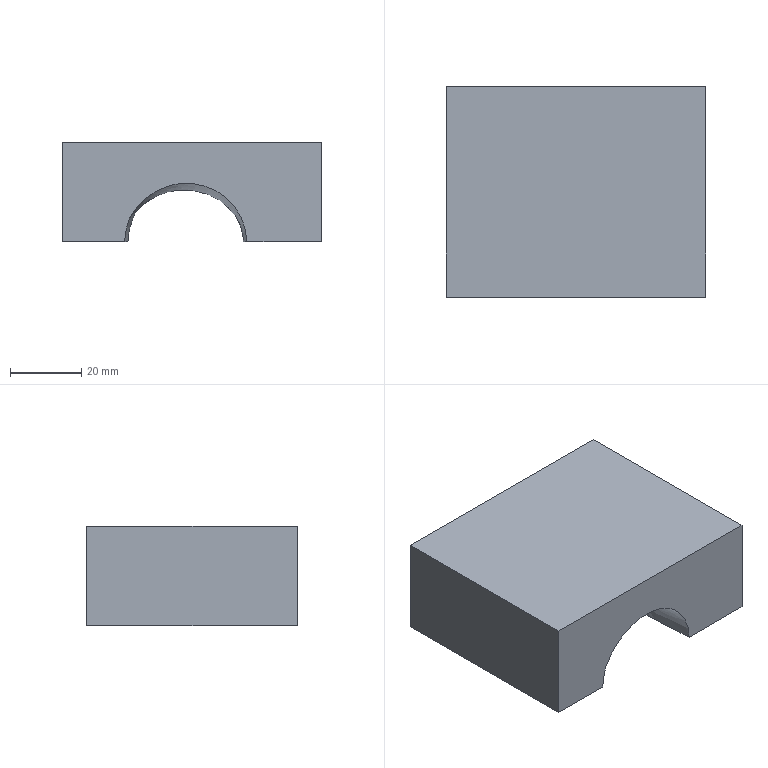NC program | NX | posted with a generic post | part box 72.744 x 59.015 x 27.972 mm
Lines 1756 to 2547 of 95982:
(FIXED_CONTOUR , TOOL : R2)
N3474 T11 M6
N3476 G54
N3478 G17 G0 G90 X13.244 Y-31.06 S9500 M3
N3480 G43 Z30. H11
N3482 Z5.2
N3484 G94 G1 Z0.147 F1000.
N3486 X13.257 Y-31.089
N3488 X13.248 Y-31.119
N3490 X13.223 Y-31.137
N3492 X13.217 Y-31.144 Z-0.024 F3000.
N3494 X13.192 Y-31.168 Z-1.496
N3496 X13.168 Y-31.192 Z-2.478
N3498 X13.124 Y-31.237 Z-3.072
N3500 X13.105 Y-31.256 Z-3.228
N3502 X13.073 Y-31.288 Z-3.473
N3504 X13.053 Y-31.289 Z-3.655
N3506 X13.028 Y-31.29 Z-3.843
N3508 X13.008 Z-3.965
N3510 X13.034 Y-31.263 Z-3.831
N3512 X13.053 Y-31.245 Z-3.714
N3514 X13.11 Y-31.188 Z-3.284
N3516 X13.134 Y-31.163 Z-3.109
N3518 X13.183 Y-31.115 Z-2.494
N3520 X13.208 Y-31.09 Z-1.499
N3522 X13.234 Y-31.064 Z0.072
N3524 X13.237 Y-31.061 Z0.149
N3526 X13.242 Y-31.031 Z0.15
N3528 X13.214 Y-31.059 Z-1.5
N3530 X13.188 Y-31.085 Z-2.501
N3532 X13.139 Y-31.134 Z-3.123
N3534 X13.087 Y-31.186 Z-3.491
N3536 X13.054 Y-31.22 Z-3.747
N3538 X13.042 Y-31.231 Z-3.817
N3540 X12.983 Y-31.29 Z-4.119
N3542 X12.959 Y-31.291 Z-4.273
N3544 X13.054 Y-31.196 Z-3.778
N3546 X13.144 Y-31.107 Z-3.135
N3548 X13.193 Y-31.057 Z-2.507
N3550 X13.219 Y-31.031 Z-1.501
N3552 X13.247 Y-31.004 Z0.151
N3554 X13.251 Y-30.981
N3556 X13.223 Y-31.009 Z-1.553
N3558 X13.198 Y-31.034 Z-2.512
N3560 X13.147 Y-31.084 Z-3.146
N3562 X13.055 Y-31.177 Z-3.799
N3564 X12.94 Y-31.292 Z-4.4
N3566 X12.921 Z-4.503
N3568 X12.947 Y-31.265 Z-4.388
N3570 X13.057 Y-31.156 Z-3.812
N3572 X13.151 Y-31.062 Z-3.156
N3574 X13.202 Y-31.011 Z-2.517
N3576 X13.229 Y-30.984 Z-1.512
N3578 X13.255 Y-30.957 Z0.152
N3580 X13.26 Y-30.933
N3582 X13.233 Y-30.96 Z-1.528
N3584 X13.206 Y-30.987 Z-2.524
N3586 X13.155 Y-31.038 Z-3.167
N3588 X13.115 Y-31.078 Z-3.449
N3590 X13.06 Y-31.133 Z-3.825
N3592 X12.957 Y-31.236 Z-4.361
N3594 X12.901 Y-31.292 Z-4.606
N3596 X12.88 Y-31.291 Z-4.713
N3598 X12.902 Y-31.27 Z-4.628
N3600 X12.969 Y-31.203 Z-4.331
N3602 X13.062 Y-31.109 Z-3.84
N3604 X13.159 Y-31.013 Z-3.179
N3606 X13.211 Y-30.96 Z-2.532
N3608 X13.238 Y-30.933 Z-1.546
N3610 X13.265 Y-30.906 Z0.153
N3612 X13.271 Y-30.877 Z0.154
N3614 X13.243 Y-30.904 Z-1.565
N3616 X13.222 Y-30.926 Z-2.383
N3618 X13.216 Y-30.932 Z-2.54
N3620 X13.162 Y-30.985 Z-3.197
N3622 X13.065 Y-31.083 Z-3.856
N3624 X12.978 Y-31.169 Z-4.312
N3626 X12.902 Y-31.246 Z-4.653
N3628 X12.89 Y-31.257 Z-4.689
N3630 X12.856 Y-31.292 Z-4.831
N3632 X12.83 Y-31.293 Z-4.96
N3634 X12.884 Y-31.238 Z-4.737
N3636 X12.902 Y-31.22 Z-4.68
N3638 X12.98 Y-31.142 Z-4.334
N3640 X13.068 Y-31.054 Z-3.873
N3642 X13.165 Y-30.957 Z-3.222
N3644 X13.172 Y-30.95 Z-3.167
N3646 X13.222 Y-30.9 Z-2.55
N3648 X13.23 Y-30.892 Z-2.32
N3650 X13.249 Y-30.873 Z-1.586
N3652 X13.277 Y-30.845 Z0.155
N3654 X13.283 Y-30.811
N3656 X13.256 Y-30.839 Z-1.608
N3658 X13.239 Y-30.856 Z-2.251
N3660 X13.228 Y-30.867 Z-2.56
N3662 X13.18 Y-30.915 Z-3.153
N3664 X13.168 Y-30.926 Z-3.25
N3666 X13.072 Y-31.023 Z-3.892
N3668 X12.982 Y-31.113 Z-4.358
N3670 X12.902 Y-31.193 Z-4.709
N3672 X12.877 Y-31.218 Z-4.789
N3674 X12.801 Y-31.293 Z-5.099
N3676 X12.768 Z-5.243
N3678 X12.802 Y-31.259 Z-5.124
N3680 X12.868 Y-31.193 Z-4.852
N3682 X12.902 Y-31.159 Z-4.744
N3684 X12.984 Y-31.078 Z-4.387
N3686 X13.08 Y-30.981 Z-3.891
N3688 X13.172 Y-30.889 Z-3.283
N3690 X13.19 Y-30.872 Z-3.137
N3692 X13.235 Y-30.826 Z-2.573
N3694 X13.249 Y-30.812 Z-2.168
N3696 X13.263 Y-30.798 Z-1.635
N3698 X13.291 Y-30.77 Z0.156
N3700 X13.298 Y-30.733 Z0.157
N3702 X13.27 Y-30.761 Z-1.66
N3704 X13.259 Y-30.773 Z-2.094
N3706 X13.242 Y-30.79 Z-2.584
N3708 X13.198 Y-30.833 Z-3.122
N3710 X13.175 Y-30.856 Z-3.312
N3712 X13.094 Y-30.938 Z-3.851
N3714 X13.078 Y-30.954 Z-3.945
N3716 X12.985 Y-31.046 Z-4.413
N3718 X12.902 Y-31.13 Z-4.772
N3720 X12.861 Y-31.171 Z-4.908
N3722 X12.802 Y-31.229 Z-5.149
N3724 X12.738 Y-31.293 Z-5.371
N3726 X12.71 Z-5.487
N3728 X12.735 Y-31.268 Z-5.408
N3730 X12.802 Y-31.201 Z-5.173
N3732 X12.854 Y-31.149 Z-4.961
N3734 X12.877 Y-31.126 Z-4.887
N3736 X12.902 Y-31.101 Z-4.799
N3738 X12.987 Y-31.016 Z-4.438
N3740 X13.08 Y-30.923 Z-3.971
N3742 X13.107 Y-30.896 Z-3.813
N3744 X13.178 Y-30.825 Z-3.341
N3746 X13.206 Y-30.797 Z-3.108
N3748 X13.248 Y-30.755 Z-2.595
N3750 X13.268 Y-30.735 Z-2.023
N3752 X13.277 Y-30.726 Z-1.683
N3754 X13.305 Y-30.698 Z0.158
N3756 X13.312 Y-30.661 Z0.159
N3758 X13.284 Y-30.689 Z-1.707
N3760 X13.277 Y-30.696 Z-1.949
N3762 X13.254 Y-30.719 Z-2.606
N3764 X13.215 Y-30.758 Z-3.093
N3766 X13.182 Y-30.791 Z-3.37
N3768 X13.121 Y-30.852 Z-3.773
N3770 X13.082 Y-30.891 Z-3.999
N3772 X12.989 Y-30.984 Z-4.464
N3774 X12.902 Y-31.071 Z-4.828
N3776 X12.866 Y-31.107 Z-4.954
N3778 X12.846 Y-31.127 Z-5.018
N3780 X12.802 Y-31.171 Z-5.198
N3782 X12.745 Y-31.228 Z-5.398
N3784 X12.702 Y-31.271 Z-5.533
N3786 X12.681 Y-31.292 Z-5.596
N3788 X12.649 Y-31.293 Z-5.712
N3790 X12.702 Y-31.239 Z-5.557
N3792 X12.755 Y-31.186 Z-5.388
N3794 X12.802 Y-31.139 Z-5.225
N3796 X12.838 Y-31.103 Z-5.078
N3798 X12.854 Y-31.087 Z-5.026
N3800 X12.902 Y-31.039 Z-4.858
N3802 X12.99 Y-30.951 Z-4.493
N3804 X13.006 Y-30.935 Z-4.42
N3806 X13.084 Y-30.857 Z-4.028
N3808 X13.136 Y-30.806 Z-3.731
N3810 X13.185 Y-30.756 Z-3.402
N3812 X13.224 Y-30.717 Z-3.077
N3814 X13.261 Y-30.68 Z-2.618
N3816 X13.287 Y-30.654 Z-1.87
N3818 X13.294 Y-30.647 Z-1.538
N3820 X13.32 Y-30.622 Z0.16
N3822 X13.328 Y-30.58 Z0.161
N3824 X13.298 Y-30.609 Z-1.786
N3826 X13.269 Y-30.639 Z-2.631
N3828 X13.234 Y-30.673 Z-3.061
N3830 X13.189 Y-30.718 Z-3.435
N3832 X13.151 Y-30.756 Z-3.686
N3834 X13.086 Y-30.821 Z-4.059
N3836 X13.019 Y-30.888 Z-4.396
N3838 X12.991 Y-30.917 Z-4.524
N3840 X12.902 Y-31.006 Z-4.89
N3842 X12.829 Y-31.078 Z-5.141
N3844 X12.802 Y-31.105 Z-5.253
N3846 X12.766 Y-31.141 Z-5.377
N3848 X12.702 Y-31.205 Z-5.582
N3850 X12.615 Y-31.293 Z-5.835
N3852 X12.579 Z-5.965
N3854 X12.702 Y-31.169 Z-5.609
N3856 X12.778 Y-31.093 Z-5.365
N3858 X12.802 Y-31.07 Z-5.283
N3860 X12.82 Y-31.052 Z-5.208
N3862 X12.911 Y-30.96 Z-4.888
N3864 X12.992 Y-30.88 Z-4.556
N3866 X13.034 Y-30.838 Z-4.37
N3868 X13.089 Y-30.783 Z-4.091
N3870 X13.168 Y-30.704 Z-3.638
N3872 X13.193 Y-30.679 Z-3.471
N3874 X13.244 Y-30.627 Z-3.043
N3876 X13.277 Y-30.595 Z-2.639
N3878 X13.301 Y-30.57 Z-2.116
N3880 X13.336 Y-30.536 Z0.161
N3882 X13.345 Y-30.487 Z0.162
N3884 X13.311 Y-30.521 Z-2.106
N3886 X13.301 Y-30.531 Z-2.374
N3888 X13.29 Y-30.542 Z-2.588
N3890 X13.257 Y-30.575 Z-3.015
N3892 X13.197 Y-30.635 Z-3.51
N3894 X13.186 Y-30.646 Z-3.585
N3896 X13.092 Y-30.74 Z-4.128
N3898 X13.049 Y-30.783 Z-4.342
N3900 X12.994 Y-30.839 Z-4.592
N3902 X12.924 Y-30.908 Z-4.875
N3904 X12.81 Y-31.022 Z-5.283
N3906 X12.792 Y-31.041 Z-5.353
N3908 X12.702 Y-31.13 Z-5.638
N3910 X12.571 Y-31.261 Z-6.016
N3912 X12.539 Y-31.293 Z-6.102
N3914 X12.497 Y-31.292 Z-6.239
N3916 X12.614 Y-31.175 Z-5.925
N3918 X12.702 Y-31.087 Z-5.67
N3920 X12.806 Y-30.984 Z-5.339
N3922 X12.939 Y-30.851 Z-4.862
N3924 X12.995 Y-30.794 Z-4.631
N3926 X13.066 Y-30.723 Z-4.312
N3928 X13.095 Y-30.694 Z-4.167
N3930 X13.205 Y-30.585 Z-3.536
N3932 X13.263 Y-30.526 Z-3.061
N3934 X13.288 Y-30.501 Z-2.764
N3936 X13.304 Y-30.485 Z-2.523
N3938 X13.322 Y-30.467 Z-2.095
N3940 X13.356 Y-30.434 Z0.163
N3942 X13.366 Y-30.38 Z0.165
N3944 X13.333 Y-30.413 Z-2.085
N3946 X13.311 Y-30.435 Z-2.581
N3948 X13.285 Y-30.461 Z-2.933
N3950 X13.266 Y-30.48 Z-3.131
N3952 X13.219 Y-30.527 Z-3.51
N3954 X13.201 Y-30.545 Z-3.621
N3956 X13.098 Y-30.648 Z-4.207
N3958 X13.083 Y-30.663 Z-4.281
N3960 X12.996 Y-30.749 Z-4.67
N3962 X12.953 Y-30.793 Z-4.848
N3964 X12.902 Y-30.844 Z-5.037
N3966 X12.82 Y-30.926 Z-5.327
N3968 X12.702 Y-31.044 Z-5.702
N3970 X12.657 Y-31.089 Z-5.832
N3972 X12.503 Y-31.243 Z-6.254
N3974 X12.483 Y-31.262 Z-6.298
N3976 X12.454 Y-31.292 Z-6.372
N3978 X12.41 Z-6.507
N3980 X12.466 Y-31.236 Z-6.367
N3982 X12.503 Y-31.199 Z-6.283
N3984 X12.702 Y-31. Z-5.735
N3986 X12.835 Y-30.867 Z-5.315
N3988 X12.902 Y-30.8 Z-5.076
N3990 X12.968 Y-30.735 Z-4.834
N3992 X12.998 Y-30.704 Z-4.709
N3994 X13.101 Y-30.602 Z-4.25
N3996 X13.201 Y-30.501 Z-3.684
N3998 X13.234 Y-30.469 Z-3.484
N4000 X13.28 Y-30.422 Z-3.101
N4002 X13.3 Y-30.402 Z-2.892
N4004 X13.32 Y-30.382 Z-2.609
N4006 X13.344 Y-30.358 Z-2.074
N4008 X13.376 Y-30.326 Z0.166
N4010 X13.387 Y-30.271 Z0.167
N4012 X13.355 Y-30.303 Z-2.063
N4014 X13.329 Y-30.329 Z-2.638
N4016 X13.315 Y-30.343 Z-2.838
N4018 X13.289 Y-30.369 Z-3.122
N4020 X13.248 Y-30.41 Z-3.458
N4022 X13.201 Y-30.457 Z-3.748
N4024 X13.115 Y-30.543 Z-4.23
N4026 X13. Y-30.659 Z-4.749
N4028 X12.982 Y-30.676 Z-4.82
N4030 X12.902 Y-30.756 Z-5.116
N4032 X12.849 Y-30.809 Z-5.302
N4034 X12.717 Y-30.942 Z-5.725
N4036 X12.503 Y-31.155 Z-6.312
N4038 X12.448 Y-31.21 Z-6.436
N4040 X12.366 Y-31.292 Z-6.642
N4042 X12.322 Z-6.779
N4044 X12.43 Y-31.184 Z-6.506
N4046 X12.503 Y-31.111 Z-6.341
N4048 X12.615 Y-30.998 Z-6.033
N4050 X12.702 Y-30.911 Z-5.799
N4052 X12.731 Y-30.882 Z-5.714
N4054 X12.802 Y-30.812 Z-5.492
N4056 X12.864 Y-30.749 Z-5.29
N4058 X12.997 Y-30.616 Z-4.805
N4060 X13.101 Y-30.512 Z-4.346
N4062 X13.13 Y-30.483 Z-4.211
N4064 X13.201 Y-30.413 Z-3.812
N4066 X13.263 Y-30.351 Z-3.432
N4068 X13.301 Y-30.313 Z-3.115
N4070 X13.329 Y-30.284 Z-2.784
N4072 X13.338 Y-30.276 Z-2.666
N4074 X13.366 Y-30.248 Z-2.052
N4076 X13.397 Y-30.216 Z0.168
N4078 X13.409 Y-30.156 Z0.169
N4080 X13.378 Y-30.187 Z-2.043
N4082 X13.346 Y-30.219 Z-2.724
N4084 X13.301 Y-30.264 Z-3.225
N4086 X13.279 Y-30.286 Z-3.403
N4088 X13.201 Y-30.364 Z-3.883
N4090 X13.146 Y-30.419 Z-4.191
N4092 X13.101 Y-30.464 Z-4.4
N4094 X13.013 Y-30.552 Z-4.789
N4096 X12.88 Y-30.685 Z-5.276
N4098 X12.802 Y-30.763 Z-5.531
N4100 X12.748 Y-30.817 Z-5.702
N4102 X12.702 Y-30.863 Z-5.834
N4104 X12.566 Y-30.998 Z-6.198
N4106 X12.503 Y-31.062 Z-6.373
N4108 X12.41 Y-31.155 Z-6.583
N4110 X12.303 Y-31.262 Z-6.852
N4112 X12.273 Y-31.292 Z-6.916
N4114 X12.226 Z-7.044
N4116 X12.303 Y-31.214 Z-6.878
N4118 X12.391 Y-31.127 Z-6.657
N4120 X12.503 Y-31.015 Z-6.404
N4122 X12.702 Y-30.815 Z-5.868
N4124 X12.763 Y-30.754 Z-5.69
N4126 X12.896 Y-30.621 Z-5.263
N4128 X13.001 Y-30.516 Z-4.879
N4130 X13.029 Y-30.488 Z-4.772
N4132 X13.101 Y-30.416 Z-4.453
N4134 X13.162 Y-30.355 Z-4.17
N4136 X13.201 Y-30.317 Z-3.951
N4138 X13.295 Y-30.223 Z-3.375
N4140 X13.301 Y-30.217 Z-3.328
N4142 X13.359 Y-30.159 Z-2.701
N4144 X13.39 Y-30.128 Z-2.045
N4146 X13.42 Y-30.098 Z0.17
N4148 X13.431 Y-30.042 Z0.171
N4150 X13.411 Y-30.062 Z-1.351
N4152 X13.401 Y-30.072 Z-2.046
N4154 X13.371 Y-30.102 Z-2.692
N4156 X13.309 Y-30.164 Z-3.356
N4158 X13.301 Y-30.172 Z-3.411
N4160 X13.201 Y-30.271 Z-4.017
N4162 X13.177 Y-30.295 Z-4.151
N4164 X13.101 Y-30.371 Z-4.504
N4166 X13.044 Y-30.428 Z-4.756
N4168 X13.001 Y-30.471 Z-4.921
N4170 X12.902 Y-30.571 Z-5.282
N4172 X12.778 Y-30.694 Z-5.679
N4174 X12.702 Y-30.77 Z-5.901
N4176 X12.503 Y-30.97 Z-6.432
N4178 X12.373 Y-31.1 Z-6.728
N4180 X12.303 Y-31.169 Z-6.902
N4182 X12.18 Y-31.292 Z-7.165
N4184 X12.136 Z-7.28
N4186 X12.178 Y-31.25 Z-7.195
N4188 X12.303 Y-31.124 Z-6.927
N4190 X12.355 Y-31.073 Z-6.798
N4192 X12.503 Y-30.925 Z-6.46
N4194 X12.576 Y-30.852 Z-6.271
N4196 X12.702 Y-30.726 Z-5.933
N4198 X12.802 Y-30.626 Z-5.64
N4200 X12.926 Y-30.502 Z-5.238
N4202 X13.001 Y-30.426 Z-4.963
N4204 X13.059 Y-30.369 Z-4.74
N4206 X13.101 Y-30.327 Z-4.554
N4208 X13.192 Y-30.236 Z-4.132
N4210 X13.301 Y-30.127 Z-3.484
N4212 X13.321 Y-30.107 Z-3.343
N4214 X13.363 Y-30.064 Z-2.899
N4216 X13.382 Y-30.046 Z-2.684
N4218 X13.412 Y-30.016 Z-2.047
N4220 X13.427 Y-30. Z-0.941
N4222 X13.441 Y-29.987 Z0.172
N4224 X13.452 Y-29.93 Z0.173
N4226 X13.435 Y-29.947 Z-1.236
N4228 X13.423 Y-29.959 Z-2.049
N4230 X13.394 Y-29.988 Z-2.676
N4232 X13.368 Y-30.014 Z-2.971
N4234 X13.334 Y-30.048 Z-3.33
N4236 X13.301 Y-30.081 Z-3.56
N4238 X13.207 Y-30.175 Z-4.112
N4240 X13.101 Y-30.281 Z-4.605
N4242 X13.074 Y-30.308 Z-4.724
N4244 X13.001 Y-30.381 Z-5.006
N4246 X12.941 Y-30.441 Z-5.225
N4248 X12.808 Y-30.574 Z-5.657
N4250 X12.702 Y-30.68 Z-5.966
N4252 X12.622 Y-30.76 Z-6.182
N4254 X12.503 Y-30.879 Z-6.488
N4256 X12.336 Y-31.046 Z-6.87
N4258 X12.303 Y-31.079 Z-6.952
N4260 X12.223 Y-31.159 Z-7.123
N4262 X12.091 Y-31.291 Z-7.393
N4264 X12.043 Y-31.292 Z-7.51
N4266 X12.08 Y-31.255 Z-7.436
N4268 X12.104 Y-31.231 Z-7.392
N4270 X12.303 Y-31.032 Z-6.978
N4272 X12.337 Y-30.998 Z-6.899
N4274 X12.503 Y-30.832 Z-6.518
N4276 X12.669 Y-30.666 Z-6.09
N4278 X12.702 Y-30.633 Z-6.
N4280 X12.824 Y-30.511 Z-5.645
N4282 X12.902 Y-30.433 Z-5.395
N4284 X12.957 Y-30.378 Z-5.212
N4286 X13.001 Y-30.334 Z-5.05
N4288 X13.09 Y-30.245 Z-4.708
N4290 X13.201 Y-30.134 Z-4.198
N4292 X13.223 Y-30.112 Z-4.09
N4294 X13.301 Y-30.035 Z-3.637
N4296 X13.347 Y-29.988 Z-3.316
N4298 X13.373 Y-29.962 Z-3.044
N4300 X13.406 Y-29.929 Z-2.667
N4302 X13.435 Y-29.9 Z-2.05
N4304 X13.463 Y-29.872 Z0.175
N4306 X13.474 Y-29.812 Z0.176
N4308 X13.447 Y-29.84 Z-2.052
N4310 X13.419 Y-29.868 Z-2.658
N4312 X13.378 Y-29.908 Z-3.121
N4314 X13.361 Y-29.926 Z-3.302
N4316 X13.301 Y-29.986 Z-3.714
N4318 X13.239 Y-30.048 Z-4.068
N4320 X13.201 Y-30.086 Z-4.255
N4322 X13.101 Y-30.186 Z-4.71
N4324 X13.001 Y-30.285 Z-5.095
N4326 X12.973 Y-30.314 Z-5.199
N4328 X12.902 Y-30.385 Z-5.435
N4330 X12.84 Y-30.447 Z-5.633
N4332 X12.702 Y-30.584 Z-6.034
N4334 X12.503 Y-30.784 Z-6.548
N4336 X12.303 Y-30.983 Z-7.005
N4338 X12.104 Y-31.183 Z-7.418
N4340 X12.06 Y-31.226 Z-7.498
N4342 X11.994 Y-31.292 Z-7.629
N4344 X11.944 Y-31.293 Z-7.752
N4346 X12.04 Y-31.197 Z-7.561
N4348 X12.104 Y-31.133 Z-7.444
N4350 X12.303 Y-30.933 Z-7.033
N4352 X12.368 Y-30.868 Z-6.888
N4354 X12.503 Y-30.734 Z-6.579
N4356 X12.638 Y-30.599 Z-6.231
N4358 X12.702 Y-30.535 Z-6.068
N4360 X12.857 Y-30.38 Z-5.621
N4362 X12.99 Y-30.247 Z-5.185
N4364 X13.123 Y-30.114 Z-4.673
N4366 X13.201 Y-30.036 Z-4.313
N4368 X13.256 Y-29.981 Z-4.045
N4370 X13.301 Y-29.936 Z-3.786
N4372 X13.375 Y-29.862 Z-3.287
N4374 X13.432 Y-29.805 Z-2.649
N4376 X13.46 Y-29.777 Z-2.046
N4378 X13.486 Y-29.751 Z0.177
N4380 X13.499 Y-29.686 Z0.178
N4382 X13.493 Y-29.691 Z-0.404
N4384 X13.473 Y-29.711 Z-2.026
N4386 X13.469 Y-29.715 Z-2.149
N4388 X13.447 Y-29.737 Z-2.625
N4390 X13.389 Y-29.795 Z-3.279
N4392 X13.301 Y-29.884 Z-3.862
N4394 X13.273 Y-29.911 Z-4.021
N4396 X13.201 Y-29.983 Z-4.375
N4398 X13.14 Y-30.044 Z-4.655
N4400 X13.101 Y-30.083 Z-4.811
N4402 X13.001 Y-30.183 Z-5.189
N4404 X12.874 Y-30.31 Z-5.608
N4406 X12.702 Y-30.482 Z-6.104
N4408 X12.585 Y-30.599 Z-6.399
N4410 X12.503 Y-30.681 Z-6.611
N4412 X12.421 Y-30.763 Z-6.8
N4414 X12.303 Y-30.881 Z-7.062
N4416 X12.104 Y-31.08 Z-7.472
N4418 X12.019 Y-31.166 Z-7.628
N4420 X11.905 Y-31.28 Z-7.855
N4422 X11.891 Y-31.293 Z-7.879
N4424 X11.837 Z-7.999
N4426 X11.905 Y-31.226 Z-7.88
N4428 X11.997 Y-31.133 Z-7.697
N4430 X12.104 Y-31.026 Z-7.501
N4432 X12.303 Y-30.827 Z-7.093
N4434 X12.503 Y-30.627 Z-6.645
N4436 X12.702 Y-30.428 Z-6.141
N4438 X12.892 Y-30.238 Z-5.595
N4440 X13.025 Y-30.105 Z-5.154
N4442 X13.101 Y-30.029 Z-4.864
N4444 X13.158 Y-29.972 Z-4.636
N4446 X13.201 Y-29.929 Z-4.439
N4448 X13.291 Y-29.839 Z-3.996
N4450 X13.301 Y-29.829 Z-3.941
N4452 X13.395 Y-29.735 Z-3.334
N4454 X13.409 Y-29.721 Z-3.221
N4456 X13.45 Y-29.68 Z-2.758
N4458 X13.462 Y-29.668 Z-2.6
N4460 X13.48 Y-29.65 Z-2.222
N4462 X13.487 Y-29.643 Z-2.006
N4464 X13.503 Y-29.627 Z-0.741
N4466 X13.512 Y-29.619 Z0.18
N4468 X13.524 Y-29.555 Z0.181
N4470 X13.512 Y-29.567 Z-1.061
N4472 X13.501 Y-29.578 Z-1.986
N4474 X13.49 Y-29.589 Z-2.291
N4476 X13.477 Y-29.602 Z-2.575
N4478 X13.459 Y-29.62 Z-2.813
N4480 X13.426 Y-29.653 Z-3.176
N4482 X13.4 Y-29.678 Z-3.386
N4484 X13.305 Y-29.774 Z-3.991
N4486 X13.201 Y-29.878 Z-4.499
N4488 X13.175 Y-29.904 Z-4.617
N4490 X13.101 Y-29.978 Z-4.914
N4492 X13.042 Y-30.037 Z-5.139
N4494 X13.001 Y-30.077 Z-5.28
N4496 X12.902 Y-30.177 Z-5.605
N4498 X12.702 Y-30.376 Z-6.177
N4500 X12.503 Y-30.576 Z-6.677
N4502 X12.303 Y-30.775 Z-7.122
N4504 X12.104 Y-30.975 Z-7.527
N4506 X11.963 Y-31.116 Z-7.788
N4508 X11.905 Y-31.174 Z-7.904
N4510 X11.786 Y-31.293 Z-8.114
N4512 X11.736 Y-31.292 Z-8.222
N4514 X11.779 Y-31.249 Z-8.149
N4516 X11.905 Y-31.124 Z-7.927
N4518 X11.955 Y-31.073 Z-7.826
N4520 X12.104 Y-30.924 Z-7.553
N4522 X12.178 Y-30.851 Z-7.406
N4524 X12.303 Y-30.725 Z-7.15
N4526 X12.503 Y-30.526 Z-6.707
N4528 X12.576 Y-30.452 Z-6.528
N4530 X12.702 Y-30.326 Z-6.211
N4532 X12.829 Y-30.2 Z-5.848
N4534 X12.902 Y-30.127 Z-5.644
N4536 X12.926 Y-30.102 Z-5.57
N4538 X13.001 Y-30.027 Z-5.323
N4540 X13.059 Y-29.969 Z-5.125
N4542 X13.101 Y-29.927 Z-4.963
N4544 X13.192 Y-29.836 Z-4.6
N4546 X13.314 Y-29.714 Z-4.01
N4548 X13.334 Y-29.694 Z-3.891
N4550 X13.406 Y-29.623 Z-3.438
N4552 X13.443 Y-29.585 Z-3.132
N4554 X13.467 Y-29.561 Z-2.866
N4556 X13.491 Y-29.537 Z-2.551
N4558 X13.5 Y-29.528 Z-2.359
N4560 X13.514 Y-29.515 Z-1.968
N4562 X13.521 Y-29.507 Z-1.375
N4564 X13.536 Y-29.493 Z0.182
N4566 X13.548 Y-29.428 Z0.183
N4568 X13.528 Y-29.449 Z-1.948
N4570 X13.511 Y-29.465 Z-2.429
N4572 X13.506 Y-29.47 Z-2.527
N4574 X13.476 Y-29.501 Z-2.921
N4576 X13.461 Y-29.515 Z-3.086
N4578 X13.411 Y-29.565 Z-3.491
N4580 X13.358 Y-29.618 Z-3.826
N4582 X13.324 Y-29.652 Z-4.03
N4584 X13.209 Y-29.767 Z-4.582
N4586 X13.076 Y-29.9 Z-5.109
N4588 X13.001 Y-29.975 Z-5.368
N4590 X12.944 Y-30.033 Z-5.558
N4592 X12.902 Y-30.075 Z-5.685
N4594 X12.776 Y-30.2 Z-6.034
N4596 X12.702 Y-30.274 Z-6.247
N4598 X12.628 Y-30.348 Z-6.433
N4600 X12.503 Y-30.473 Z-6.738
N4602 X12.303 Y-30.673 Z-7.179
N4604 X12.23 Y-30.746 Z-7.329
N4606 X12.104 Y-30.872 Z-7.579
N4608 X11.934 Y-31.042 Z-7.893
N4610 X11.905 Y-31.072 Z-7.952
N4612 X11.831 Y-31.145 Z-8.081
N4614 X11.685 Y-31.292 Z-8.327
N4616 X11.63 Z-8.436
N4618 X11.705 Y-31.217 Z-8.318
N4620 X11.905 Y-31.018 Z-7.977
N4622 X12.104 Y-30.818 Z-7.607
N4624 X12.303 Y-30.619 Z-7.21
N4626 X12.503 Y-30.42 Z-6.771
N4628 X12.702 Y-30.22 Z-6.284
N4630 X12.902 Y-30.021 Z-5.726
N4632 X12.961 Y-29.961 Z-5.545
N4634 X13.001 Y-29.921 Z-5.414
N4636 X13.101 Y-29.821 Z-5.068
N4638 X13.227 Y-29.695 Z-4.565
N4640 X13.334 Y-29.588 Z-4.051
N4642 X13.383 Y-29.539 Z-3.759
N4644 X13.417 Y-29.505 Z-3.546
N4646 X13.479 Y-29.443 Z-3.039
N4648 X13.522 Y-29.401 Z-2.501
N4650 X13.541 Y-29.381 Z-1.948
N4652 X13.561 Y-29.362 Z0.185
N4654 X13.574 Y-29.293 Z0.186
N4656 X13.562 Y-29.305 Z-0.98
N4658 X13.554 Y-29.313 Z-1.996
N4660 X13.538 Y-29.329 Z-2.449
N4662 X13.534 Y-29.333 Z-2.529
N4664 X13.496 Y-29.37 Z-3.008
N4666 X13.423 Y-29.444 Z-3.602
N4668 X13.345 Y-29.522 Z-4.073
N4670 X13.246 Y-29.621 Z-4.548
N4672 X13.201 Y-29.666 Z-4.731
N4674 X13.113 Y-29.754 Z-5.078
N4676 X12.98 Y-29.887 Z-5.532
N4678 X12.902 Y-29.965 Z-5.769
N4680 X12.738 Y-30.129 Z-6.226
N4682 X12.702 Y-30.164 Z-6.321
N4684 X12.503 Y-30.364 Z-6.804
N4686 X12.303 Y-30.563 Z-7.24
N4688 X12.104 Y-30.763 Z-7.635
N4690 X11.905 Y-30.962 Z-8.003
N4692 X11.705 Y-31.162 Z-8.343
N4694 X11.653 Y-31.213 Z-8.422
N4696 X11.574 Y-31.292 Z-8.549
N4698 X11.516 Y-31.293 Z-8.665
N4700 X11.63 Y-31.179 Z-8.483
N4702 X11.705 Y-31.104 Z-8.368
N4704 X11.811 Y-30.998 Z-8.187
N4706 X11.905 Y-30.905 Z-8.031
N4708 X12.104 Y-30.705 Z-7.664
N4710 X12.303 Y-30.506 Z-7.271
N4712 X12.397 Y-30.413 Z-7.073
N4714 X12.503 Y-30.306 Z-6.839
N4716 X12.609 Y-30.2 Z-6.58
N4718 X12.702 Y-30.107 Z-6.359
N4720 X12.795 Y-30.014 Z-6.111
N4722 X12.902 Y-29.908 Z-5.813
N4724 X13.001 Y-29.808 Z-5.511
N4726 X13.132 Y-29.677 Z-5.062
N4728 X13.201 Y-29.608 Z-4.79
N4730 X13.265 Y-29.544 Z-4.529
N4732 X13.355 Y-29.454 Z-4.095
N4734 X13.434 Y-29.376 Z-3.626
N4736 X13.5 Y-29.309 Z-3.101
N4738 X13.511 Y-29.298 Z-3.001
N4740 X13.546 Y-29.263 Z-2.558
N4742 X13.555 Y-29.255 Z-2.397
N4744 X13.567 Y-29.243 Z-2.046
N4746 X13.569 Y-29.241 Z-1.65
N4748 X13.58 Y-29.229 Z-0.425
N4750 X13.587 Y-29.222 Z0.187
N4752 X13.602 Y-29.145 Z0.189
N4754 X13.591 Y-29.156 Z-0.687
N4756 X13.584 Y-29.163 Z-1.514
N4758 X13.581 Y-29.166 Z-2.1
N4760 X13.573 Y-29.174 Z-2.339
N4762 X13.559 Y-29.188 Z-2.589
N4764 X13.528 Y-29.219 Z-2.993
N4766 X13.508 Y-29.239 Z-3.17
N4768 X13.457 Y-29.29 Z-3.575
N4770 X13.369 Y-29.378 Z-4.107
N4772 X13.286 Y-29.461 Z-4.51
N4774 X13.201 Y-29.546 Z-4.855
N4776 X13.153 Y-29.594 Z-5.045
N4778 X13.101 Y-29.646 Z-5.227
N4780 X13.02 Y-29.727 Z-5.504
N4782 X12.902 Y-29.845 Z-5.862
N4784 X12.857 Y-29.89 Z-5.986
N4786 X12.702 Y-30.045 Z-6.4
N4788 X12.503 Y-30.244 Z-6.877
N4790 X12.459 Y-30.288 Z-6.974
N4792 X12.303 Y-30.444 Z-7.304
N4794 X12.104 Y-30.643 Z-7.696
N4796 X11.905 Y-30.842 Z-8.062
N4798 X11.705 Y-31.042 Z-8.395
N4800 X11.605 Y-31.142 Z-8.549
N4802 X11.506 Y-31.241 Z-8.708
N4804 X11.454 Y-31.293 Z-8.782
N4806 X11.394 Y-31.292 Z-8.895
N4808 X11.506 Y-31.18 Z-8.733
N4810 X11.58 Y-31.106 Z-8.614
N4812 X11.723 Y-30.963 Z-8.393
N4814 X11.905 Y-30.781 Z-8.091
N4816 X12.121 Y-30.564 Z-7.693
N4818 X12.303 Y-30.382 Z-7.337
N4820 X12.503 Y-30.183 Z-6.913
N4822 X12.702 Y-29.983 Z-6.44
N4824 X12.902 Y-29.784 Z-5.908
N4826 X13.04 Y-29.646 Z-5.49
N4828 X13.101 Y-29.585 Z-5.282
N4830 X13.173 Y-29.513 Z-5.029
N4832 X13.305 Y-29.381 Z-4.496
N4834 X13.388 Y-29.298 Z-4.091
N4836 X13.423 Y-29.263 Z-3.866
N4838 X13.479 Y-29.207 Z-3.524
N4840 X13.515 Y-29.171 Z-3.237
N4842 X13.544 Y-29.142 Z-2.985
N4844 X13.572 Y-29.113 Z-2.62
N4846 X13.59 Y-29.095 Z-2.283
N4848 X13.595 Y-29.091 Z-2.153
N4850 X13.599 Y-29.087 Z-1.38
N4852 X13.603 Y-29.083 Z-0.943
N4854 X13.617 Y-29.069 Z0.19
N4856 X13.631 Y-28.996 Z0.192
N4858 X13.613 Y-29.014 Z-1.251
N4860 X13.607 Y-29.019 Z-2.229
N4862 X13.585 Y-29.042 Z-2.649
N4864 X13.559 Y-29.068 Z-2.978
N4866 X13.523 Y-29.104 Z-3.301
N4868 X13.5 Y-29.127 Z-3.476
N4870 X13.466 Y-29.161 Z-3.684
N4872 X13.405 Y-29.222 Z-4.076
N4874 X13.319 Y-29.308 Z-4.5
N4876 X13.301 Y-29.326 Z-4.58
N4878 X13.193 Y-29.434 Z-5.012
N4880 X13.101 Y-29.526 Z-5.335
N4882 X13.06 Y-29.567 Z-5.476
N4884 X12.902 Y-29.725 Z-5.952
N4886 X12.826 Y-29.801 Z-6.148
N4888 X12.702 Y-29.925 Z-6.479
N4890 X12.579 Y-30.048 Z-6.774
N4892 X12.503 Y-30.124 Z-6.947
N4894 X12.303 Y-30.324 Z-7.368
N4896 X12.104 Y-30.523 Z-7.756
N4898 X11.905 Y-30.722 Z-8.12
N4900 X11.782 Y-30.845 Z-8.324
N4902 X11.705 Y-30.922 Z-8.448
N4904 X11.556 Y-31.071 Z-8.676
N4906 X11.506 Y-31.121 Z-8.757
N4908 X11.335 Y-31.292 Z-9.004
N4910 X11.277 Z-9.108
N4912 X11.306 Y-31.263 Z-9.069
N4914 X11.506 Y-31.063 Z-8.78
N4916 X11.705 Y-30.864 Z-8.473
N4918 X11.84 Y-30.729 Z-8.256
N4920 X11.905 Y-30.664 Z-8.148
N4922 X12.104 Y-30.465 Z-7.786
N4924 X12.303 Y-30.265 Z-7.4
N4926 X12.503 Y-30.066 Z-6.981
N4928 X12.637 Y-29.932 Z-6.674
N4930 X12.702 Y-29.866 Z-6.518
N4932 X12.768 Y-29.801 Z-6.342
N4934 X12.902 Y-29.667 Z-5.994
N4936 X13.079 Y-29.49 Z-5.462
N4938 X13.212 Y-29.357 Z-4.996
N4940 X13.301 Y-29.268 Z-4.645
N4942 X13.333 Y-29.236 Z-4.503
N4944 X13.423 Y-29.146 Z-4.061
N4946 X13.522 Y-29.047 Z-3.428
N4948 X13.574 Y-28.995 Z-2.973
N4950 X13.597 Y-28.971 Z-2.668
N4952 X13.622 Y-28.947 Z-2.213
N4954 X13.627 Y-28.942 Z-1.241
N4956 X13.644 Y-28.924 Z0.193
N4958 X13.659 Y-28.851 Z0.195
N4960 X13.64 Y-28.869 Z-1.254
N4962 X13.635 Y-28.874 Z-2.209
N4964 X13.61 Y-28.899 Z-2.673
N4966 X13.585 Y-28.924 Z-2.988
N4968 X13.538 Y-28.971 Z-3.412
N4970 X13.441 Y-29.069 Z-4.045
N4972 X13.347 Y-29.162 Z-4.506
N4974 X13.294 Y-29.215 Z-4.739
N4976 X13.232 Y-29.277 Z-4.978
N4978 X13.099 Y-29.41 Z-5.448
N4980 X12.902 Y-29.607 Z-6.038
N4982 X12.696 Y-29.813 Z-6.572
N4984 X12.503 Y-30.006 Z-7.015
N4986 X12.298 Y-30.212 Z-7.443
N4988 X12.104 Y-30.405 Z-7.815
N4990 X11.899 Y-30.61 Z-8.186
N4992 X11.705 Y-30.804 Z-8.499
N4994 X11.506 Y-31.004 Z-8.805
N4996 X11.306 Y-31.203 Z-9.093
N4998 X11.217 Y-31.292 Z-9.21
N5000 X11.157 Z-9.314
N5002 X11.306 Y-31.142 Z-9.118
N5004 X11.506 Y-30.943 Z-8.83
N5006 X11.705 Y-30.743 Z-8.526
N5008 X11.905 Y-30.544 Z-8.205
N5010 X12.104 Y-30.345 Z-7.846
N5012 X12.303 Y-30.145 Z-7.464
N5014 X12.503 Y-29.946 Z-7.05
N5016 X12.702 Y-29.746 Z-6.596
N5018 X12.757 Y-29.692 Z-6.46
N5020 X12.902 Y-29.547 Z-6.083
N5022 X13.101 Y-29.347 Z-5.49
N5024 X13.119 Y-29.329 Z-5.433
N5026 X13.252 Y-29.196 Z-4.96
N5028 X13.301 Y-29.148 Z-4.773
N5030 X13.362 Y-29.087 Z-4.51
N5032 X13.459 Y-28.99 Z-4.03
N5034 X13.548 Y-28.901 Z-3.437
N5036 X13.565 Y-28.884 Z-3.3
N5038 X13.597 Y-28.851 Z-3.004
N5040 X13.623 Y-28.826 Z-2.679
N5042 X13.649 Y-28.799 Z-2.204
N5044 X13.654 Y-28.794 Z-1.268
N5046 X13.668 Y-28.78 Z-0.066
N5048 X13.673 Y-28.776 Z0.196
N5050 X13.688 Y-28.699 Z0.197